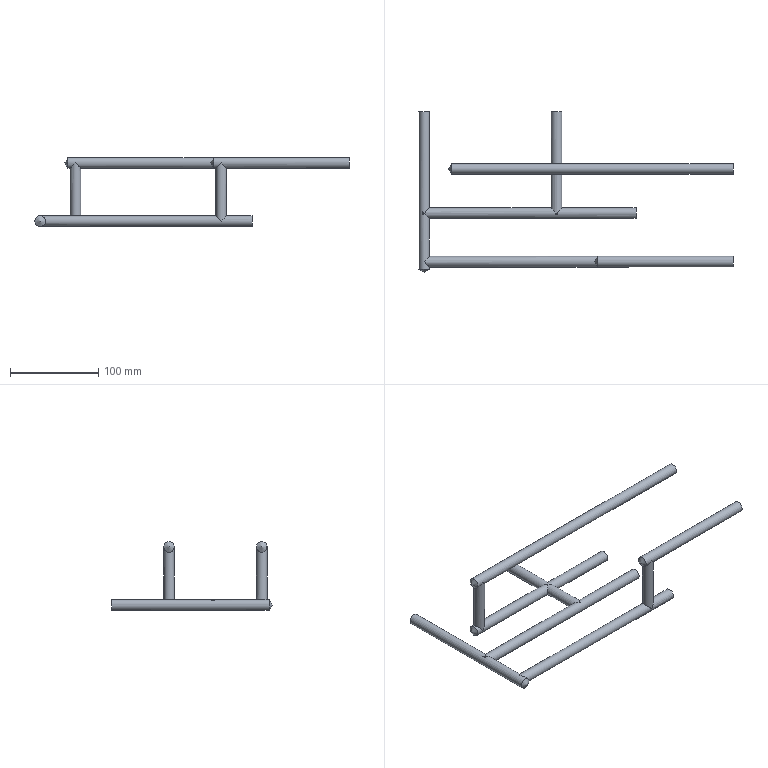Part | STEP file | SOLID | 1 solid | 30 faces | box 356 x 182.01 x 78 mm | volume 174730 mm3 | cylinder 15 | plane 11 | cone 4 | commonest cylinder face diameters 12 x15